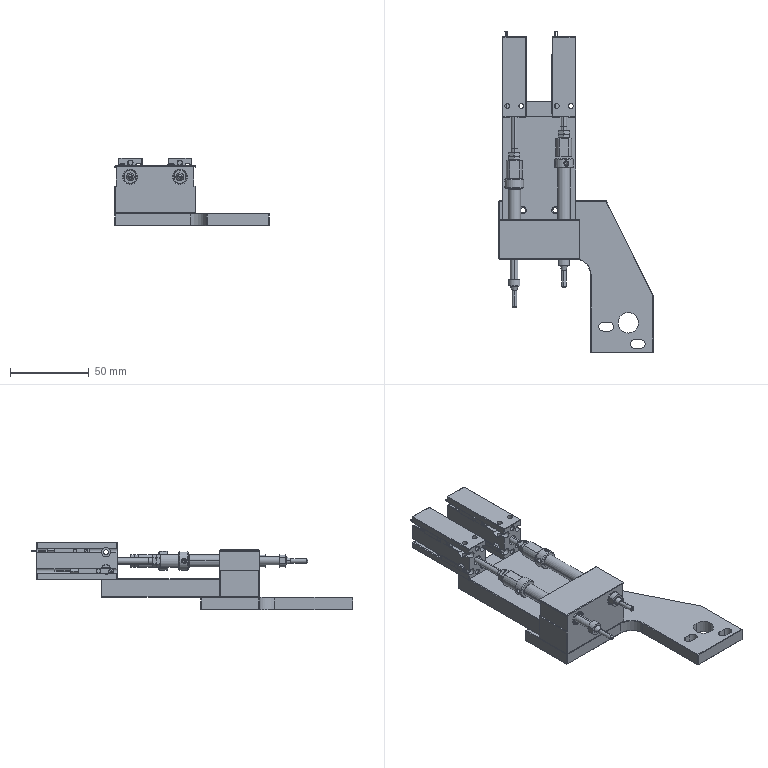Part | NX | 29 solids | 1130 faces | box 98.5 x 204.4 x 43.237 mm | volume 150636 mm3 | cylinder 435 | plane 353 | cone 202 | torus 108 | sphere 16 | spline 16 | commonest cylinder face diameters 0.5 x56 4 x44 5 x40 3.2 x32 3.3 x28 6 x28